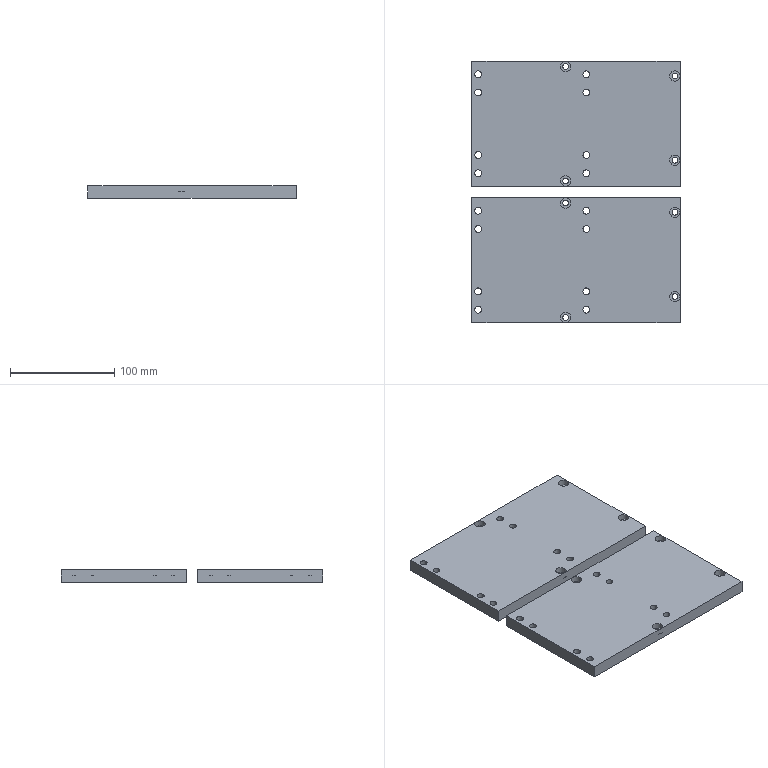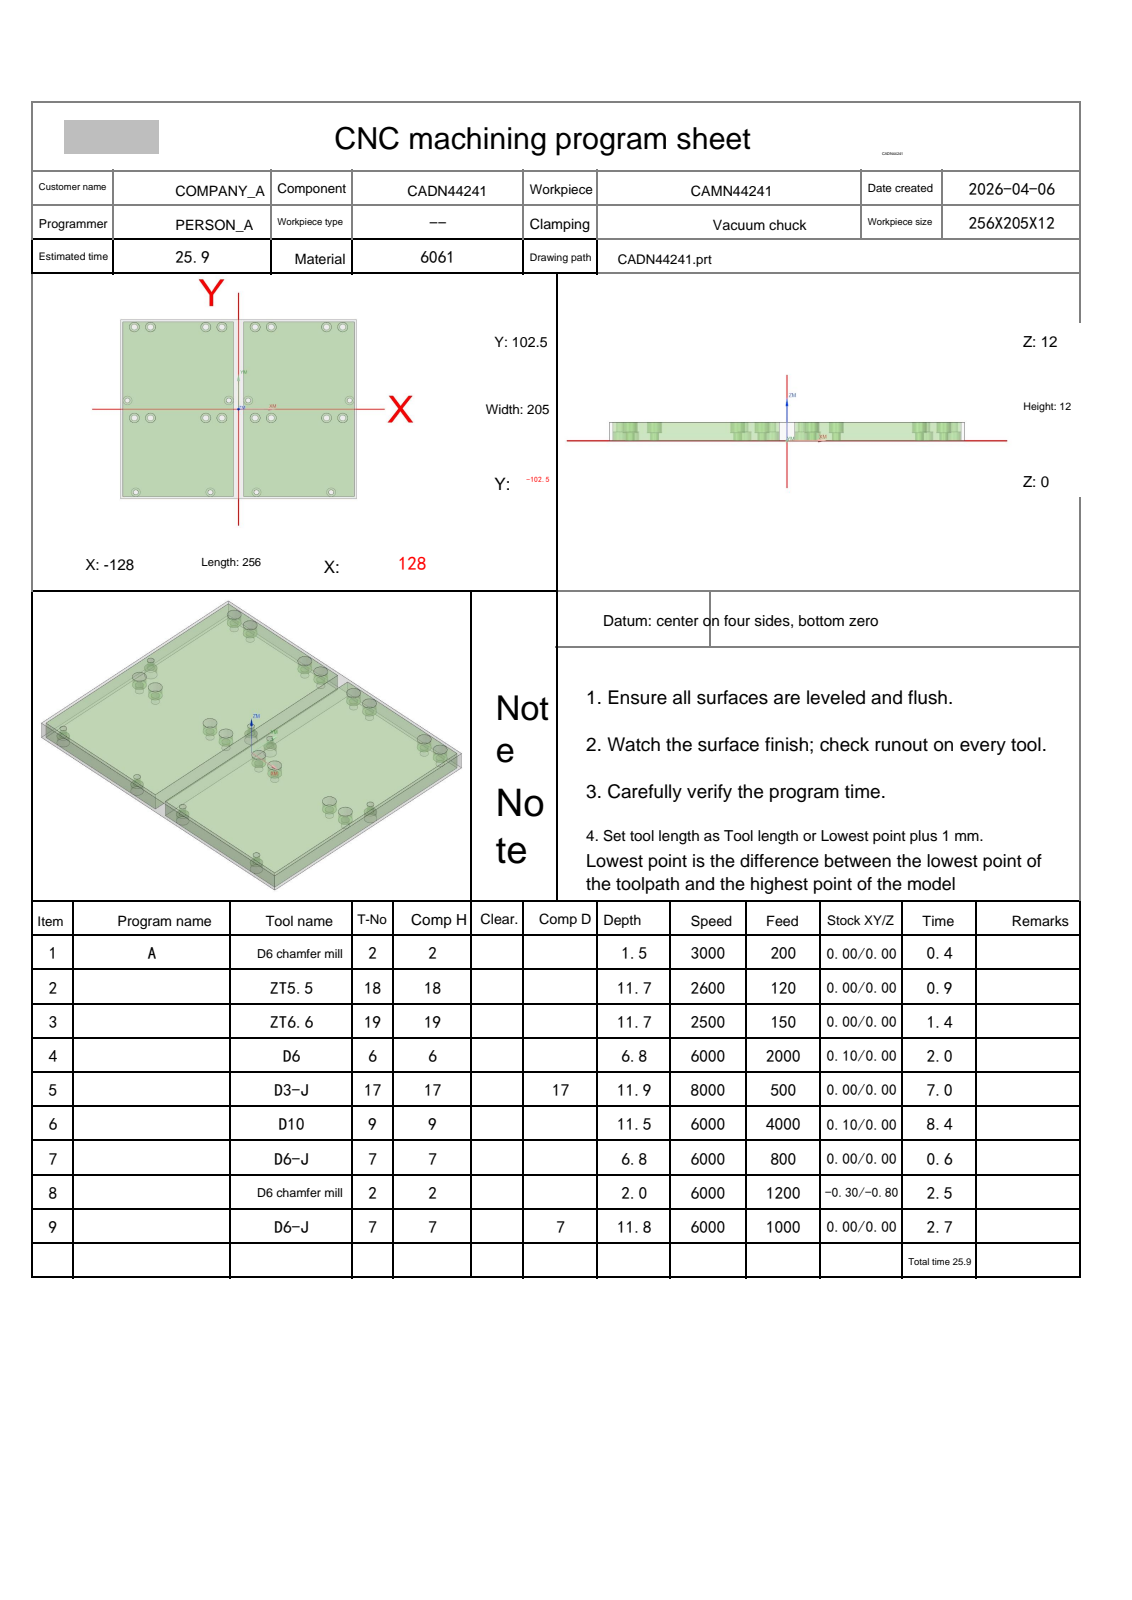NC program | NX | posted by the shop | part box 200 x 251 x 12 mm
Lines 2394 to 3499 of 3499:
N6 T09 M06
(D10  D=10. R=0. H=09 ce=0.10 di=0.00)
G00 G90 G54 X-130.6 Y0.0 M03 S6000
G43 H09 Z32.
M08
Z12.5
G01 Y100. Z12.426 F4000.
G02 X-125.5 Y105.1 Z12.42 I5.1 J0.0
G01 X-5.5 Z12.33
G02 X-.4 Y100. Z12.324 I0.0 J-5.1
G01 Y-100. Z12.176
G02 X-5.5 Y-105.1 Z12.17 I-5.1 J0.0
G01 X-125.5 Z12.08
G02 X-130.6 Y-100. Z12.074 I0.0 J5.1
G01 Y100. Z11.926
G02 X-125.5 Y105.1 Z11.92 I5.1 J0.0
G01 X-5.5 Z11.83
G02 X-.4 Y100. Z11.824 I0.0 J-5.1
G01 Y-100. Z11.676
G02 X-5.5 Y-105.1 Z11.67 I-5.1 J0.0
G01 X-125.5 Z11.58
G02 X-130.6 Y-100. Z11.574 I0.0 J5.1
G01 Y100. Z11.426
G02 X-125.5 Y105.1 Z11.42 I5.1 J0.0
G01 X-5.5 Z11.33
G02 X-.4 Y100. Z11.324 I0.0 J-5.1
G01 Y-100. Z11.176
G02 X-5.5 Y-105.1 Z11.17 I-5.1 J0.0
G01 X-125.5 Z11.08
G02 X-130.6 Y-100. Z11.074 I0.0 J5.1
G01 Y100. Z10.926
G02 X-125.5 Y105.1 Z10.92 I5.1 J0.0
G01 X-5.5 Z10.83
G02 X-.4 Y100. Z10.824 I0.0 J-5.1
G01 Y-100. Z10.676
G02 X-5.5 Y-105.1 Z10.67 I-5.1 J0.0
G01 X-125.5 Z10.58
G02 X-130.6 Y-100. Z10.574 I0.0 J5.1
G01 Y100. Z10.426
G02 X-125.5 Y105.1 Z10.42 I5.1 J0.0
G01 X-5.5 Z10.33
G02 X-.4 Y100. Z10.324 I0.0 J-5.1
G01 Y-100. Z10.176
G02 X-5.5 Y-105.1 Z10.17 I-5.1 J0.0
G01 X-125.5 Z10.08
G02 X-130.6 Y-100. Z10.074 I0.0 J5.1
G01 Y100. Z9.926
G02 X-125.5 Y105.1 Z9.92 I5.1 J0.0
G01 X-5.5 Z9.83
G02 X-.4 Y100. Z9.824 I0.0 J-5.1
G01 Y-100. Z9.676
G02 X-5.5 Y-105.1 Z9.67 I-5.1 J0.0
G01 X-125.5 Z9.58
G02 X-130.6 Y-100. Z9.574 I0.0 J5.1
G01 Y100. Z9.426
G02 X-125.5 Y105.1 Z9.42 I5.1 J0.0
G01 X-5.5 Z9.33
G02 X-.4 Y100. Z9.324 I0.0 J-5.1
G01 Y-100. Z9.176
G02 X-5.5 Y-105.1 Z9.17 I-5.1 J0.0
G01 X-125.5 Z9.08
G02 X-130.6 Y-100. Z9.074 I0.0 J5.1
G01 Y100. Z8.926
G02 X-125.5 Y105.1 Z8.92 I5.1 J0.0
G01 X-5.5 Z8.83
G02 X-.4 Y100. Z8.824 I0.0 J-5.1
G01 Y-100. Z8.676
G02 X-5.5 Y-105.1 Z8.67 I-5.1 J0.0
G01 X-125.5 Z8.58
G02 X-130.6 Y-100. Z8.574 I0.0 J5.1
G01 Y100. Z8.426
G02 X-125.5 Y105.1 Z8.42 I5.1 J0.0
G01 X-5.5 Z8.33
G02 X-.4 Y100. Z8.324 I0.0 J-5.1
G01 Y-100. Z8.176
G02 X-5.5 Y-105.1 Z8.17 I-5.1 J0.0
G01 X-125.5 Z8.08
G02 X-130.6 Y-100. Z8.074 I0.0 J5.1
G01 Y100. Z7.926
G02 X-125.5 Y105.1 Z7.92 I5.1 J0.0
G01 X-5.5 Z7.83
G02 X-.4 Y100. Z7.824 I0.0 J-5.1
G01 Y-100. Z7.676
G02 X-5.5 Y-105.1 Z7.67 I-5.1 J0.0
G01 X-125.5 Z7.58
G02 X-130.6 Y-100. Z7.574 I0.0 J5.1
G01 Y100. Z7.426
G02 X-125.5 Y105.1 Z7.42 I5.1 J0.0
G01 X-5.5 Z7.33
G02 X-.4 Y100. Z7.324 I0.0 J-5.1
G01 Y-100. Z7.176
G02 X-5.5 Y-105.1 Z7.17 I-5.1 J0.0
G01 X-125.5 Z7.08
G02 X-130.6 Y-100. Z7.074 I0.0 J5.1
G01 Y100. Z6.926
G02 X-125.5 Y105.1 Z6.92 I5.1 J0.0
G01 X-5.5 Z6.83
G02 X-.4 Y100. Z6.824 I0.0 J-5.1
G01 Y-100. Z6.676
G02 X-5.5 Y-105.1 Z6.67 I-5.1 J0.0
G01 X-125.5 Z6.58
G02 X-130.6 Y-100. Z6.574 I0.0 J5.1
G01 Y100. Z6.426
G02 X-125.5 Y105.1 Z6.42 I5.1 J0.0
G01 X-5.5 Z6.33
G02 X-.4 Y100. Z6.324 I0.0 J-5.1
G01 Y-100. Z6.176
G02 X-5.5 Y-105.1 Z6.17 I-5.1 J0.0
G01 X-125.5 Z6.08
G02 X-130.6 Y-100. Z6.074 I0.0 J5.1
G01 Y100. Z5.926
G02 X-125.5 Y105.1 Z5.92 I5.1 J0.0
G01 X-5.5 Z5.83
G02 X-.4 Y100. Z5.824 I0.0 J-5.1
G01 Y-100. Z5.676
G02 X-5.5 Y-105.1 Z5.67 I-5.1 J0.0
G01 X-125.5 Z5.58
G02 X-130.6 Y-100. Z5.574 I0.0 J5.1
G01 Y100. Z5.426
G02 X-125.5 Y105.1 Z5.42 I5.1 J0.0
G01 X-5.5 Z5.33
G02 X-.4 Y100. Z5.324 I0.0 J-5.1
G01 Y-100. Z5.176
G02 X-5.5 Y-105.1 Z5.17 I-5.1 J0.0
G01 X-125.5 Z5.08
G02 X-130.6 Y-100. Z5.074 I0.0 J5.1
G01 Y100. Z4.926
G02 X-125.5 Y105.1 Z4.92 I5.1 J0.0
G01 X-5.5 Z4.83
G02 X-.4 Y100. Z4.824 I0.0 J-5.1
G01 Y-100. Z4.676
G02 X-5.5 Y-105.1 Z4.67 I-5.1 J0.0
G01 X-125.5 Z4.58
G02 X-130.6 Y-100. Z4.574 I0.0 J5.1
G01 Y100. Z4.426
G02 X-125.5 Y105.1 Z4.42 I5.1 J0.0
G01 X-5.5 Z4.33
G02 X-.4 Y100. Z4.324 I0.0 J-5.1
G01 Y-100. Z4.176
G02 X-5.5 Y-105.1 Z4.17 I-5.1 J0.0
G01 X-125.5 Z4.08
G02 X-130.6 Y-100. Z4.074 I0.0 J5.1
G01 Y100. Z3.926
G02 X-125.5 Y105.1 Z3.92 I5.1 J0.0
G01 X-5.5 Z3.83
G02 X-.4 Y100. Z3.824 I0.0 J-5.1
G01 Y-100. Z3.676
G02 X-5.5 Y-105.1 Z3.67 I-5.1 J0.0
G01 X-125.5 Z3.58
G02 X-130.6 Y-100. Z3.574 I0.0 J5.1
G01 Y100. Z3.426
G02 X-125.5 Y105.1 Z3.42 I5.1 J0.0
G01 X-5.5 Z3.33
G02 X-.4 Y100. Z3.324 I0.0 J-5.1
G01 Y-100. Z3.176
G02 X-5.5 Y-105.1 Z3.17 I-5.1 J0.0
G01 X-125.5 Z3.08
G02 X-130.6 Y-100. Z3.074 I0.0 J5.1
G01 Y100. Z2.926
G02 X-125.5 Y105.1 Z2.92 I5.1 J0.0
G01 X-5.5 Z2.83
G02 X-.4 Y100. Z2.824 I0.0 J-5.1
G01 Y-100. Z2.676
G02 X-5.5 Y-105.1 Z2.67 I-5.1 J0.0
G01 X-125.5 Z2.58
G02 X-130.6 Y-100. Z2.574 I0.0 J5.1
G01 Y100. Z2.426
G02 X-125.5 Y105.1 Z2.42 I5.1 J0.0
G01 X-5.5 Z2.33
G02 X-.4 Y100. Z2.324 I0.0 J-5.1
G01 Y-100. Z2.176
G02 X-5.5 Y-105.1 Z2.17 I-5.1 J0.0
G01 X-125.5 Z2.08
G02 X-130.6 Y-100. Z2.074 I0.0 J5.1
G01 Y100. Z1.926
G02 X-125.5 Y105.1 Z1.92 I5.1 J0.0
G01 X-5.5 Z1.83
G02 X-.4 Y100. Z1.824 I0.0 J-5.1
G01 Y-100. Z1.676
G02 X-5.5 Y-105.1 Z1.67 I-5.1 J0.0
G01 X-125.5 Z1.58
G02 X-130.6 Y-100. Z1.574 I0.0 J5.1
G01 Y100. Z1.426
G02 X-125.5 Y105.1 Z1.42 I5.1 J0.0
G01 X-5.5 Z1.33
G02 X-.4 Y100. Z1.324 I0.0 J-5.1
G01 Y-100. Z1.176
G02 X-5.5 Y-105.1 Z1.17 I-5.1 J0.0
G01 X-125.5 Z1.08
G02 X-130.6 Y-100. Z1.074 I0.0 J5.1
G01 Y100. Z.926
G02 X-125.5 Y105.1 Z.92 I5.1 J0.0
G01 X-5.5 Z.83
G02 X-.4 Y100. Z.824 I0.0 J-5.1
G01 Y-100. Z.676
G02 X-5.5 Y-105.1 Z.67 I-5.1 J0.0
G01 X-125.5 Z.58
G02 X-130.6 Y-100. Z.574 I0.0 J5.1
G01 Y0.0 Z.5
Y100.
G02 X-125.5 Y105.1 I5.1 J0.0
G01 X-5.5
G02 X-.4 Y100. I0.0 J-5.1
G01 Y-100.
G02 X-5.5 Y-105.1 I-5.1 J0.0
G01 X-125.5
G02 X-130.6 Y-100. I0.0 J5.1
G01 Y0.0
Y.5
Z1.5
G00 Z32.
X130.6 Y0.0
Z12.5
G01 Y-100. Z12.426
G02 X125.5 Y-105.1 Z12.42 I-5.1 J0.0
G01 X5.5 Z12.33
G02 X.4 Y-100. Z12.324 I0.0 J5.1
G01 Y100. Z12.176
G02 X5.5 Y105.1 Z12.17 I5.1 J0.0
G01 X125.5 Z12.08
G02 X130.6 Y100. Z12.074 I0.0 J-5.1
G01 Y-100. Z11.926
G02 X125.5 Y-105.1 Z11.92 I-5.1 J0.0
G01 X5.5 Z11.83
G02 X.4 Y-100. Z11.824 I0.0 J5.1
G01 Y100. Z11.676
G02 X5.5 Y105.1 Z11.67 I5.1 J0.0
G01 X125.5 Z11.58
G02 X130.6 Y100. Z11.574 I0.0 J-5.1
G01 Y-100. Z11.426
G02 X125.5 Y-105.1 Z11.42 I-5.1 J0.0
G01 X5.5 Z11.33
G02 X.4 Y-100. Z11.324 I0.0 J5.1
G01 Y100. Z11.176
G02 X5.5 Y105.1 Z11.17 I5.1 J0.0
G01 X125.5 Z11.08
G02 X130.6 Y100. Z11.074 I0.0 J-5.1
G01 Y-100. Z10.926
G02 X125.5 Y-105.1 Z10.92 I-5.1 J0.0
G01 X5.5 Z10.83
G02 X.4 Y-100. Z10.824 I0.0 J5.1
G01 Y100. Z10.676
G02 X5.5 Y105.1 Z10.67 I5.1 J0.0
G01 X125.5 Z10.58
G02 X130.6 Y100. Z10.574 I0.0 J-5.1
G01 Y-100. Z10.426
G02 X125.5 Y-105.1 Z10.42 I-5.1 J0.0
G01 X5.5 Z10.33
G02 X.4 Y-100. Z10.324 I0.0 J5.1
G01 Y100. Z10.176
G02 X5.5 Y105.1 Z10.17 I5.1 J0.0
G01 X125.5 Z10.08
G02 X130.6 Y100. Z10.074 I0.0 J-5.1
G01 Y-100. Z9.926
G02 X125.5 Y-105.1 Z9.92 I-5.1 J0.0
G01 X5.5 Z9.83
G02 X.4 Y-100. Z9.824 I0.0 J5.1
G01 Y100. Z9.676
G02 X5.5 Y105.1 Z9.67 I5.1 J0.0
G01 X125.5 Z9.58
G02 X130.6 Y100. Z9.574 I0.0 J-5.1
G01 Y-100. Z9.426
G02 X125.5 Y-105.1 Z9.42 I-5.1 J0.0
G01 X5.5 Z9.33
G02 X.4 Y-100. Z9.324 I0.0 J5.1
G01 Y100. Z9.176
G02 X5.5 Y105.1 Z9.17 I5.1 J0.0
G01 X125.5 Z9.08
G02 X130.6 Y100. Z9.074 I0.0 J-5.1
G01 Y-100. Z8.926
G02 X125.5 Y-105.1 Z8.92 I-5.1 J0.0
G01 X5.5 Z8.83
G02 X.4 Y-100. Z8.824 I0.0 J5.1
G01 Y100. Z8.676
G02 X5.5 Y105.1 Z8.67 I5.1 J0.0
G01 X125.5 Z8.58
G02 X130.6 Y100. Z8.574 I0.0 J-5.1
G01 Y-100. Z8.426
G02 X125.5 Y-105.1 Z8.42 I-5.1 J0.0
G01 X5.5 Z8.33
G02 X.4 Y-100. Z8.324 I0.0 J5.1
G01 Y100. Z8.176
G02 X5.5 Y105.1 Z8.17 I5.1 J0.0
G01 X125.5 Z8.08
G02 X130.6 Y100. Z8.074 I0.0 J-5.1
G01 Y-100. Z7.926
G02 X125.5 Y-105.1 Z7.92 I-5.1 J0.0
G01 X5.5 Z7.83
G02 X.4 Y-100. Z7.824 I0.0 J5.1
G01 Y100. Z7.676
G02 X5.5 Y105.1 Z7.67 I5.1 J0.0
G01 X125.5 Z7.58
G02 X130.6 Y100. Z7.574 I0.0 J-5.1
G01 Y-100. Z7.426
G02 X125.5 Y-105.1 Z7.42 I-5.1 J0.0
G01 X5.5 Z7.33
G02 X.4 Y-100. Z7.324 I0.0 J5.1
G01 Y100. Z7.176
G02 X5.5 Y105.1 Z7.17 I5.1 J0.0
G01 X125.5 Z7.08
G02 X130.6 Y100. Z7.074 I0.0 J-5.1
G01 Y-100. Z6.926
G02 X125.5 Y-105.1 Z6.92 I-5.1 J0.0
G01 X5.5 Z6.83
G02 X.4 Y-100. Z6.824 I0.0 J5.1
G01 Y100. Z6.676
G02 X5.5 Y105.1 Z6.67 I5.1 J0.0
G01 X125.5 Z6.58
G02 X130.6 Y100. Z6.574 I0.0 J-5.1
G01 Y-100. Z6.426
G02 X125.5 Y-105.1 Z6.42 I-5.1 J0.0
G01 X5.5 Z6.33
G02 X.4 Y-100. Z6.324 I0.0 J5.1
G01 Y100. Z6.176
G02 X5.5 Y105.1 Z6.17 I5.1 J0.0
G01 X125.5 Z6.08
G02 X130.6 Y100. Z6.074 I0.0 J-5.1
G01 Y-100. Z5.926
G02 X125.5 Y-105.1 Z5.92 I-5.1 J0.0
G01 X5.5 Z5.83
G02 X.4 Y-100. Z5.824 I0.0 J5.1
G01 Y100. Z5.676
G02 X5.5 Y105.1 Z5.67 I5.1 J0.0
G01 X125.5 Z5.58
G02 X130.6 Y100. Z5.574 I0.0 J-5.1
G01 Y-100. Z5.426
G02 X125.5 Y-105.1 Z5.42 I-5.1 J0.0
G01 X5.5 Z5.33
G02 X.4 Y-100. Z5.324 I0.0 J5.1
G01 Y100. Z5.176
G02 X5.5 Y105.1 Z5.17 I5.1 J0.0
G01 X125.5 Z5.08
G02 X130.6 Y100. Z5.074 I0.0 J-5.1
G01 Y-100. Z4.926
G02 X125.5 Y-105.1 Z4.92 I-5.1 J0.0
G01 X5.5 Z4.83
G02 X.4 Y-100. Z4.824 I0.0 J5.1
G01 Y100. Z4.676
G02 X5.5 Y105.1 Z4.67 I5.1 J0.0
G01 X125.5 Z4.58
G02 X130.6 Y100. Z4.574 I0.0 J-5.1
G01 Y-100. Z4.426
G02 X125.5 Y-105.1 Z4.42 I-5.1 J0.0
G01 X5.5 Z4.33
G02 X.4 Y-100. Z4.324 I0.0 J5.1
G01 Y100. Z4.176
G02 X5.5 Y105.1 Z4.17 I5.1 J0.0
G01 X125.5 Z4.08
G02 X130.6 Y100. Z4.074 I0.0 J-5.1
G01 Y-100. Z3.926
G02 X125.5 Y-105.1 Z3.92 I-5.1 J0.0
G01 X5.5 Z3.83
G02 X.4 Y-100. Z3.824 I0.0 J5.1
G01 Y100. Z3.676
G02 X5.5 Y105.1 Z3.67 I5.1 J0.0
G01 X125.5 Z3.58
G02 X130.6 Y100. Z3.574 I0.0 J-5.1
G01 Y-100. Z3.426
G02 X125.5 Y-105.1 Z3.42 I-5.1 J0.0
G01 X5.5 Z3.33
G02 X.4 Y-100. Z3.324 I0.0 J5.1
G01 Y100. Z3.176
G02 X5.5 Y105.1 Z3.17 I5.1 J0.0
G01 X125.5 Z3.08
G02 X130.6 Y100. Z3.074 I0.0 J-5.1
G01 Y-100. Z2.926
G02 X125.5 Y-105.1 Z2.92 I-5.1 J0.0
G01 X5.5 Z2.83
G02 X.4 Y-100. Z2.824 I0.0 J5.1
G01 Y100. Z2.676
G02 X5.5 Y105.1 Z2.67 I5.1 J0.0
G01 X125.5 Z2.58
G02 X130.6 Y100. Z2.574 I0.0 J-5.1
G01 Y-100. Z2.426
G02 X125.5 Y-105.1 Z2.42 I-5.1 J0.0
G01 X5.5 Z2.33
G02 X.4 Y-100. Z2.324 I0.0 J5.1
G01 Y100. Z2.176
G02 X5.5 Y105.1 Z2.17 I5.1 J0.0
G01 X125.5 Z2.08
G02 X130.6 Y100. Z2.074 I0.0 J-5.1
G01 Y-100. Z1.926
G02 X125.5 Y-105.1 Z1.92 I-5.1 J0.0
G01 X5.5 Z1.83
G02 X.4 Y-100. Z1.824 I0.0 J5.1
G01 Y100. Z1.676
G02 X5.5 Y105.1 Z1.67 I5.1 J0.0
G01 X125.5 Z1.58
G02 X130.6 Y100. Z1.574 I0.0 J-5.1
G01 Y-100. Z1.426
G02 X125.5 Y-105.1 Z1.42 I-5.1 J0.0
G01 X5.5 Z1.33
G02 X.4 Y-100. Z1.324 I0.0 J5.1
G01 Y100. Z1.176
G02 X5.5 Y105.1 Z1.17 I5.1 J0.0
G01 X125.5 Z1.08
G02 X130.6 Y100. Z1.074 I0.0 J-5.1
G01 Y-100. Z.926
G02 X125.5 Y-105.1 Z.92 I-5.1 J0.0
G01 X5.5 Z.83
G02 X.4 Y-100. Z.824 I0.0 J5.1
G01 Y100. Z.676
G02 X5.5 Y105.1 Z.67 I5.1 J0.0
G01 X125.5 Z.58
G02 X130.6 Y100. Z.574 I0.0 J-5.1
G01 Y0.0 Z.5
Y-100.
G02 X125.5 Y-105.1 I-5.1 J0.0
G01 X5.5
G02 X.4 Y-100. I0.0 J5.1
G01 Y100.
G02 X5.5 Y105.1 I5.1 J0.0
G01 X125.5
G02 X130.6 Y100. I0.0 J-5.1
G01 Y0.0
Y-.5
Z1.5
G00 Z32.
G91 G28 Z0.0
M05
M09
G91 G28 Z0.0
M01
N7 T07 M06
(D6-J  D=6. R=0. H=07 ce=0.00 di=0.00)
G00 G90 G54 X18. Y94. M03 S6000
G43 H07 Z32.
M08
Z5.2
G01 X17.638 Y91.932 F800.
X17.632 Y91.868
G03 X18. Y91.5 I.368 J0.0
X20.5 Y94. I0.0 J2.5
X18. Y96.5 I-2.5 J0.0
X15.5 Y94. I0.0 J-2.5
X18. Y91.5 I2.5 J0.0
X18.497 Y91.55 I0.0 J2.5
X18.792 Y91.91 I-.073 J.361
G01 X18.766 Y92.045
X18. Y94.
G00 Z32.
X35.5
Z5.2
G01 X35.138 Y91.932
X35.132 Y91.868
G03 X35.5 Y91.5 I.368 J0.0
X38. Y94. I0.0 J2.5
X35.5 Y96.5 I-2.5 J0.0
X33. Y94. I0.0 J-2.5
X35.5 Y91.5 I2.5 J0.0
X35.997 Y91.55 I0.0 J2.5
X36.292 Y91.91 I-.073 J.361
G01 X36.266 Y92.045
X35.5 Y94.
G00 Z32.
X-18.
Z5.2
G01 X-18.362 Y91.932
X-18.368 Y91.868
G03 X-18. Y91.5 I.368 J0.0
X-15.5 Y94. I0.0 J2.5
X-18. Y96.5 I-2.5 J0.0
X-20.5 Y94. I0.0 J-2.5
X-18. Y91.5 I2.5 J0.0
X-17.503 Y91.55 I0.0 J2.5
X-17.208 Y91.91 I-.073 J.361
G01 X-17.234 Y92.045
X-18. Y94.
G00 Z32.
X-35.5
Z5.2
G01 X-35.862 Y91.932
X-35.868 Y91.868
G03 X-35.5 Y91.5 I.368 J0.0
X-33. Y94. I0.0 J2.5
X-35.5 Y96.5 I-2.5 J0.0
X-38. Y94. I0.0 J-2.5
X-35.5 Y91.5 I2.5 J0.0
X-35.003 Y91.55 I0.0 J2.5
X-34.708 Y91.91 I-.073 J.361
G01 X-34.734 Y92.045
X-35.5 Y94.
G00 Z32.
X-95.5
Z5.2
G01 X-95.862 Y91.932
X-95.868 Y91.868
G03 X-95.5 Y91.5 I.368 J0.0
X-93. Y94. I0.0 J2.5
X-95.5 Y96.5 I-2.5 J0.0
X-98. Y94. I0.0 J-2.5
X-95.5 Y91.5 I2.5 J0.0
X-95.003 Y91.55 I0.0 J2.5
X-94.708 Y91.91 I-.073 J.361
G01 X-94.734 Y92.045
X-95.5 Y94.
G00 Z32.
X-113.
Z5.2
G01 X-113.362 Y91.932
X-113.368 Y91.868
G03 X-113. Y91.5 I.368 J0.0
X-110.5 Y94. I0.0 J2.5
X-113. Y96.5 I-2.5 J0.0
X-115.5 Y94. I0.0 J-2.5
X-113. Y91.5 I2.5 J0.0
X-112.503 Y91.55 I0.0 J2.5
X-112.208 Y91.91 I-.073 J.361
G01 X-112.234 Y92.045
X-113. Y94.
G00 Z32.
Y-10.
Z5.2
G01 X-113.362 Y-12.068
X-113.368 Y-12.132
G03 X-113. Y-12.5 I.368 J0.0
X-110.5 Y-10. I0.0 J2.5
X-113. Y-7.5 I-2.5 J0.0
X-115.5 Y-10. I0.0 J-2.5
X-113. Y-12.5 I2.5 J0.0
X-112.503 Y-12.45 I0.0 J2.5
X-112.208 Y-12.09 I-.073 J.361
G01 X-112.234 Y-11.955
X-113. Y-10.
G00 Z32.
X-95.5
Z5.2
G01 X-95.862 Y-12.068
X-95.868 Y-12.132
G03 X-95.5 Y-12.5 I.368 J0.0
X-93. Y-10. I0.0 J2.5
X-95.5 Y-7.5 I-2.5 J0.0
X-98. Y-10. I0.0 J-2.5
X-95.5 Y-12.5 I2.5 J0.0
X-95.003 Y-12.45 I0.0 J2.5
X-94.708 Y-12.09 I-.073 J.361
G01 X-94.734 Y-11.955
X-95.5 Y-10.
G00 Z32.
X-35.5
Z5.2
G01 X-35.862 Y-12.068
X-35.868 Y-12.132
G03 X-35.5 Y-12.5 I.368 J0.0
X-33. Y-10. I0.0 J2.5
X-35.5 Y-7.5 I-2.5 J0.0
X-38. Y-10. I0.0 J-2.5
X-35.5 Y-12.5 I2.5 J0.0
X-35.003 Y-12.45 I0.0 J2.5
X-34.708 Y-12.09 I-.073 J.361
G01 X-34.734 Y-11.955
X-35.5 Y-10.
G00 Z32.
X-18.
Z5.2
G01 X-18.362 Y-12.068
X-18.368 Y-12.132
G03 X-18. Y-12.5 I.368 J0.0
X-15.5 Y-10. I0.0 J2.5
X-18. Y-7.5 I-2.5 J0.0
X-20.5 Y-10. I0.0 J-2.5
X-18. Y-12.5 I2.5 J0.0
X-17.503 Y-12.45 I0.0 J2.5
X-17.208 Y-12.09 I-.073 J.361
G01 X-17.234 Y-11.955
X-18. Y-10.
G00 Z32.
X18.
Z5.2
G01 X17.638 Y-12.068
X17.632 Y-12.132
G03 X18. Y-12.5 I.368 J0.0
X20.5 Y-10. I0.0 J2.5
X18. Y-7.5 I-2.5 J0.0
X15.5 Y-10. I0.0 J-2.5
X18. Y-12.5 I2.5 J0.0
X18.497 Y-12.45 I0.0 J2.5
X18.792 Y-12.09 I-.073 J.361
G01 X18.766 Y-11.955
X18. Y-10.
G00 Z32.
X35.5
Z5.2
G01 X35.138 Y-12.068
X35.132 Y-12.132
G03 X35.5 Y-12.5 I.368 J0.0
X38. Y-10. I0.0 J2.5
X35.5 Y-7.5 I-2.5 J0.0
X33. Y-10. I0.0 J-2.5
X35.5 Y-12.5 I2.5 J0.0
X35.997 Y-12.45 I0.0 J2.5
X36.292 Y-12.09 I-.073 J.361
G01 X36.266 Y-11.955
X35.5 Y-10.
G00 Z32.
X95.5
Z5.2
G01 X95.138 Y-12.068
X95.132 Y-12.132
G03 X95.5 Y-12.5 I.368 J0.0
X98. Y-10. I0.0 J2.5
X95.5 Y-7.5 I-2.5 J0.0
X93. Y-10. I0.0 J-2.5
X95.5 Y-12.5 I2.5 J0.0
X95.997 Y-12.45 I0.0 J2.5
X96.292 Y-12.09 I-.073 J.361
G01 X96.266 Y-11.955
X95.5 Y-10.
G00 Z32.
X113.
Z5.2
G01 X112.638 Y-12.068
X112.632 Y-12.132
G03 X113. Y-12.5 I.368 J0.0
X115.5 Y-10. I0.0 J2.5
X113. Y-7.5 I-2.5 J0.0
X110.5 Y-10. I0.0 J-2.5
X113. Y-12.5 I2.5 J0.0
X113.497 Y-12.45 I0.0 J2.5
X113.792 Y-12.09 I-.073 J.361
G01 X113.766 Y-11.955
X113. Y-10.
G00 Z32.
Y94.
Z5.2
G01 X112.638 Y91.932
X112.632 Y91.868
G03 X113. Y91.5 I.368 J0.0
X115.5 Y94. I0.0 J2.5
X113. Y96.5 I-2.5 J0.0
X110.5 Y94. I0.0 J-2.5
X113. Y91.5 I2.5 J0.0
X113.497 Y91.55 I0.0 J2.5
X113.792 Y91.91 I-.073 J.361
G01 X113.766 Y92.045
X113. Y94.
G00 Z32.
X95.5
Z5.2
G01 X95.138 Y91.932
X95.132 Y91.868
G03 X95.5 Y91.5 I.368 J0.0
X98. Y94. I0.0 J2.5
X95.5 Y96.5 I-2.5 J0.0
X93. Y94. I0.0 J-2.5
X95.5 Y91.5 I2.5 J0.0
X95.997 Y91.55 I0.0 J2.5
X96.292 Y91.91 I-.073 J.361
G01 X96.266 Y92.045
X95.5 Y94.
G00 Z32.
G91 G28 Z0.0
M05
M09
G91 G28 Z0.0
M01
N8 T02 M06
(D6 chamfer mill  D=6. R=0. H=02 ce=0.00 di=0.00)
G00 G90 G54 X-3.372 Y.25 M03 S6000
G43 H02 Z32.
M08
Z14.099
G01 Z10.5 F1200.
G03 X-3.672 Y.33 I-.3 J-.52
X-4.192 Y.03 I0.0 J-.6
G01 X-4.2 Y0.0
Y-100.
G02 X-5.5 Y-101.3 I-1.3 J0.0
G01 X-125.5
G02 X-126.8 Y-100. I0.0 J1.3
G01 Y100.
G02 X-125.5 Y101.3 I1.3 J0.0
G01 X-5.5
G02 X-4.2 Y100. I0.0 J-1.3
G01 Y0.0
X-4.192 Y-.03
G03 X-3.672 Y-.33 I.52 J.3
X-3.372 Y-.25 I0.0 J.6
G01 Z14.099
G00 Z14.25
X3.372
Z14.099
G01 Z10.5
G03 X3.672 Y-.33 I.3 J.52
X4.192 Y-.03 I0.0 J.6
G01 X4.2 Y0.0
Y100.
G02 X5.5 Y101.3 I1.3 J0.0
G01 X125.5
G02 X126.8 Y100. I0.0 J-1.3
G01 Y-100.
G02 X125.5 Y-101.3 I-1.3 J0.0
G01 X5.5
G02 X4.2 Y-100. I0.0 J1.3
G01 Y0.0
X4.192 Y.03
G03 X3.672 Y.33 I-.52 J-.3
X3.372 Y.25 I0.0 J-.6
G01 Z14.099
G00 Z32.
G00 G90 X-9.853 Y10.065 M03 S6000
Z32.
Z11.1
G01 Z10.6 F600.
X-9. Y10.15
G03 X-10.5 Y11.65 I-1.5 J0.0
X-12.15 Y10. I0.0 J-1.65
X-10.5 Y8.35 I1.65 J0.0
X-8.85 Y10. I0.0 J1.65
X-10.5 Y11.65 I-1.65 J0.0
X-12. Y10.15 I0.0 J-1.5
G01 X-11.147 Y10.065
Z11.1
G00 Z32.
X11.147
Z11.1
G01 Z10.6
X12. Y10.15
G03 X10.5 Y11.65 I-1.5 J0.0
X8.85 Y10. I0.0 J-1.65
X10.5 Y8.35 I1.65 J0.0
X12.15 Y10. I0.0 J1.65
X10.5 Y11.65 I-1.65 J0.0
X9. Y10.15 I0.0 J-1.5
G01 X9.853 Y10.065
Z11.1
G00 Z32.
X121.147
Z11.1
G01 Z10.6
X122. Y10.15
G03 X120.5 Y11.65 I-1.5 J0.0
X118.85 Y10. I0.0 J-1.65
X120.5 Y8.35 I1.65 J0.0
X122.15 Y10. I0.0 J1.65
X120.5 Y11.65 I-1.65 J0.0
X119. Y10.15 I0.0 J-1.5
G01 X119.853 Y10.065
Z11.1
G00 Z32.
X101.147 Y-94.935
Z11.1
G01 Z10.6
X102. Y-94.85
G03 X100.5 Y-93.35 I-1.5 J0.0
X98.85 Y-95. I0.0 J-1.65
X100.5 Y-96.65 I1.65 J0.0
X102.15 Y-95. I0.0 J1.65
X100.5 Y-93.35 I-1.65 J0.0
X99. Y-94.85 I0.0 J-1.5
G01 X99.853 Y-94.935
Z11.1
G00 Z32.
X20.147
Z11.1
G01 Z10.6
X21. Y-94.85
G03 X19.5 Y-93.35 I-1.5 J0.0
X17.85 Y-95. I0.0 J-1.65
X19.5 Y-96.65 I1.65 J0.0
X21.15 Y-95. I0.0 J1.65
X19.5 Y-93.35 I-1.65 J0.0
X18. Y-94.85 I0.0 J-1.5
G01 X18.853 Y-94.935
Z11.1
G00 Z32.
X-29.853
Z11.1
G01 Z10.6
X-29. Y-94.85
G03 X-30.5 Y-93.35 I-1.5 J0.0
X-32.15 Y-95. I0.0 J-1.65
X-30.5 Y-96.65 I1.65 J0.0
X-28.85 Y-95. I0.0 J1.65
X-30.5 Y-93.35 I-1.65 J0.0
X-32. Y-94.85 I0.0 J-1.5
G01 X-31.147 Y-94.935
Z11.1
G00 Z32.
X-110.853
Z11.1
G01 Z10.6
X-110. Y-94.85
G03 X-111.5 Y-93.35 I-1.5 J0.0
X-113.15 Y-95. I0.0 J-1.65
X-111.5 Y-96.65 I1.65 J0.0
X-109.85 Y-95. I0.0 J1.65
X-111.5 Y-93.35 I-1.65 J0.0
X-113. Y-94.85 I0.0 J-1.5
G01 X-112.147 Y-94.935
Z11.1
G00 Z32.
X-119.853 Y10.065
Z11.1
G01 Z10.6
X-119. Y10.15
G03 X-120.5 Y11.65 I-1.5 J0.0
X-122.15 Y10. I0.0 J-1.65
X-120.5 Y8.35 I1.65 J0.0
X-118.85 Y10. I0.0 J1.65
X-120.5 Y11.65 I-1.65 J0.0
X-122. Y10.15 I0.0 J-1.5
G01 X-121.147 Y10.065
Z11.1
G00 Z32.
G00 G90 X115.705 Y94.721 M03 S6000
Z32.
Z10.5
G01 Z10. F600.
X116. Y94.8
G03 X113. Y97.8 I-3. J0.0
X109.2 Y94. I0.0 J-3.8
X113. Y90.2 I3.8 J0.0
X116.8 Y94. I0.0 J3.8
X113. Y97.8 I-3.8 J0.0
X110. Y94.8 I0.0 J-3.
G01 X110.295 Y94.721
Z10.5
G00 Z32.
X98.205
Z10.5
G01 Z10.
X98.5 Y94.8
G03 X95.5 Y97.8 I-3. J0.0
X91.7 Y94. I0.0 J-3.8
X95.5 Y90.2 I3.8 J0.0
X99.3 Y94. I0.0 J3.8
X95.5 Y97.8 I-3.8 J0.0
X92.5 Y94.8 I0.0 J-3.
G01 X92.795 Y94.721
Z10.5
G00 Z32.
X38.205
Z10.5
G01 Z10.
X38.5 Y94.8
G03 X35.5 Y97.8 I-3. J0.0
X31.7 Y94. I0.0 J-3.8
X35.5 Y90.2 I3.8 J0.0
X39.3 Y94. I0.0 J3.8
X35.5 Y97.8 I-3.8 J0.0
X32.5 Y94.8 I0.0 J-3.
G01 X32.795 Y94.721
Z10.5
G00 Z32.
X20.705
Z10.5
G01 Z10.
X21. Y94.8
G03 X18. Y97.8 I-3. J0.0
X14.2 Y94. I0.0 J-3.8
X18. Y90.2 I3.8 J0.0
X21.8 Y94. I0.0 J3.8
X18. Y97.8 I-3.8 J0.0
X15. Y94.8 I0.0 J-3.
G01 X15.295 Y94.721
Z10.5
G00 Z32.
X-15.295
Z10.5
G01 Z10.
X-15. Y94.8
G03 X-18. Y97.8 I-3. J0.0
X-21.8 Y94. I0.0 J-3.8
X-18. Y90.2 I3.8 J0.0
X-14.2 Y94. I0.0 J3.8
X-18. Y97.8 I-3.8 J0.0
X-21. Y94.8 I0.0 J-3.
G01 X-20.705 Y94.721
Z10.5
G00 Z32.
X-32.795
Z10.5
G01 Z10.
X-32.5 Y94.8
G03 X-35.5 Y97.8 I-3. J0.0
X-39.3 Y94. I0.0 J-3.8
X-35.5 Y90.2 I3.8 J0.0
X-31.7 Y94. I0.0 J3.8
X-35.5 Y97.8 I-3.8 J0.0
X-38.5 Y94.8 I0.0 J-3.
G01 X-38.205 Y94.721
Z10.5
G00 Z32.
X-92.795
Z10.5
G01 Z10.
X-92.5 Y94.8
G03 X-95.5 Y97.8 I-3. J0.0
X-99.3 Y94. I0.0 J-3.8
X-95.5 Y90.2 I3.8 J0.0
X-91.7 Y94. I0.0 J3.8
X-95.5 Y97.8 I-3.8 J0.0
X-98.5 Y94.8 I0.0 J-3.
G01 X-98.205 Y94.721
Z10.5
G00 Z32.
X-110.295
Z10.5
G01 Z10.
X-110. Y94.8
G03 X-113. Y97.8 I-3. J0.0
X-116.8 Y94. I0.0 J-3.8
X-113. Y90.2 I3.8 J0.0
X-109.2 Y94. I0.0 J3.8
X-113. Y97.8 I-3.8 J0.0
X-116. Y94.8 I0.0 J-3.
G01 X-115.705 Y94.721
Z10.5
G00 Z32.
X-110.295 Y-9.279
Z10.5
G01 Z10.
X-110. Y-9.2
G03 X-113. Y-6.2 I-3. J0.0
X-116.8 Y-10. I0.0 J-3.8
X-113. Y-13.8 I3.8 J0.0
X-109.2 Y-10. I0.0 J3.8
X-113. Y-6.2 I-3.8 J0.0
X-116. Y-9.2 I0.0 J-3.
G01 X-115.705 Y-9.279
Z10.5
G00 Z32.
X-92.795
Z10.5
G01 Z10.
X-92.5 Y-9.2
G03 X-95.5 Y-6.2 I-3. J0.0
X-99.3 Y-10. I0.0 J-3.8
X-95.5 Y-13.8 I3.8 J0.0
X-91.7 Y-10. I0.0 J3.8
X-95.5 Y-6.2 I-3.8 J0.0
X-98.5 Y-9.2 I0.0 J-3.
G01 X-98.205 Y-9.279
Z10.5
G00 Z32.
X-32.795
Z10.5
G01 Z10.
X-32.5 Y-9.2
G03 X-35.5 Y-6.2 I-3. J0.0
X-39.3 Y-10. I0.0 J-3.8
X-35.5 Y-13.8 I3.8 J0.0
X-31.7 Y-10. I0.0 J3.8
X-35.5 Y-6.2 I-3.8 J0.0
X-38.5 Y-9.2 I0.0 J-3.
G01 X-38.205 Y-9.279
Z10.5
G00 Z32.
X-15.295
Z10.5
G01 Z10.
X-15. Y-9.2
G03 X-18. Y-6.2 I-3. J0.0
X-21.8 Y-10. I0.0 J-3.8
X-18. Y-13.8 I3.8 J0.0
X-14.2 Y-10. I0.0 J3.8
X-18. Y-6.2 I-3.8 J0.0
X-21. Y-9.2 I0.0 J-3.
G01 X-20.705 Y-9.279
Z10.5
G00 Z32.
X20.705
Z10.5
G01 Z10.
X21. Y-9.2
G03 X18. Y-6.2 I-3. J0.0
X14.2 Y-10. I0.0 J-3.8
X18. Y-13.8 I3.8 J0.0
X21.8 Y-10. I0.0 J3.8
X18. Y-6.2 I-3.8 J0.0
X15. Y-9.2 I0.0 J-3.
G01 X15.295 Y-9.279
Z10.5
G00 Z32.
X38.205
Z10.5
G01 Z10.
X38.5 Y-9.2
G03 X35.5 Y-6.2 I-3. J0.0
X31.7 Y-10. I0.0 J-3.8
X35.5 Y-13.8 I3.8 J0.0
X39.3 Y-10. I0.0 J3.8
X35.5 Y-6.2 I-3.8 J0.0
X32.5 Y-9.2 I0.0 J-3.
G01 X32.795 Y-9.279
Z10.5
G00 Z32.
X98.205
Z10.5
G01 Z10.
X98.5 Y-9.2
G03 X95.5 Y-6.2 I-3. J0.0
X91.7 Y-10. I0.0 J-3.8
X95.5 Y-13.8 I3.8 J0.0
X99.3 Y-10. I0.0 J3.8
X95.5 Y-6.2 I-3.8 J0.0
X92.5 Y-9.2 I0.0 J-3.
G01 X92.795 Y-9.279
Z10.5
G00 Z32.
X115.705
Z10.5
G01 Z10.
X116. Y-9.2
G03 X113. Y-6.2 I-3. J0.0
X109.2 Y-10. I0.0 J-3.8
X113. Y-13.8 I3.8 J0.0
X116.8 Y-10. I0.0 J3.8
X113. Y-6.2 I-3.8 J0.0
X110. Y-9.2 I0.0 J-3.
G01 X110.295 Y-9.279
Z10.5
G00 Z32.
G91 G28 Z0.0
M05
M09
G91 G28 Z0.0
M01
N9 T07 M06
(D6-J  D=6. R=0. H=07 ce=0.00 di=0.00)
G00 G90 G54 X129.573 Y101.017 M03 S6000
G43 H07 Z32.
M08
Z1.
G01 Z.5 F1000.
G41 D07
X129.375 Y100.992
G03 X128.5 Y100. I.125 J-.992
G01 Y-100.
G02 X125.5 Y-103. I-3. J0.0
G01 X5.5
G02 X2.5 Y-100. I0.0 J3.
G01 Y100.
G02 X5.5 Y103. I3. J0.0
G01 X125.5
G02 X128.5 Y100. I0.0 J-3.
G01 Y99.5
G03 X129.5 Y98.5 I1. J0.0
G01 G40 X129.7
Z1.
G00 Z32.
X-129.573 Y-101.017
Z1.
G01 Z.5
G41 D07
X-129.375 Y-100.992
G03 X-128.5 Y-100. I-.125 J.992
G01 Y100.
G02 X-125.5 Y103. I3. J0.0
G01 X-5.5
G02 X-2.5 Y100. I0.0 J-3.
G01 Y-100.
G02 X-5.5 Y-103. I-3. J0.0
G01 X-125.5
G02 X-128.5 Y-100. I0.0 J3.
G01 Y-99.5
G03 X-129.5 Y-98.5 I-1. J0.0
G01 G40 X-129.7
Z1.
G00 Z32.
G00 G90 X129.474 Y101.005 M03 S6000
Z32.
Z.7
G01 Z.2 F1000.
G41 D07
X129.375 Y100.992
G03 X128.5 Y100. I.125 J-.992
G01 Y-100.
G02 X125.5 Y-103. I-3. J0.0
G01 X5.5
G02 X2.5 Y-100. I0.0 J3.
G01 Y100.
G02 X5.5 Y103. I3. J0.0
G01 X125.5
G02 X128.5 Y100. I0.0 J-3.
G01 Y99.5
G03 X129.5 Y98.5 I1. J0.0
G01 G40 X129.6
Z.7
G00 Z32.
X-129.474 Y-101.005
Z.7
G01 Z.2
G41 D07
X-129.375 Y-100.992
G03 X-128.5 Y-100. I-.125 J.992
G01 Y100.
G02 X-125.5 Y103. I3. J0.0
G01 X-5.5
G02 X-2.5 Y100. I0.0 J-3.
G01 Y-100.
G02 X-5.5 Y-103. I-3. J0.0
G01 X-125.5
G02 X-128.5 Y-100. I0.0 J3.
G01 Y-99.5
G03 X-129.5 Y-98.5 I-1. J0.0
G01 G40 X-129.6
Z.7
G00 Z32.
M05
M09
G91 G28 Z0.0
G91 G28 Y0.0
M30
%